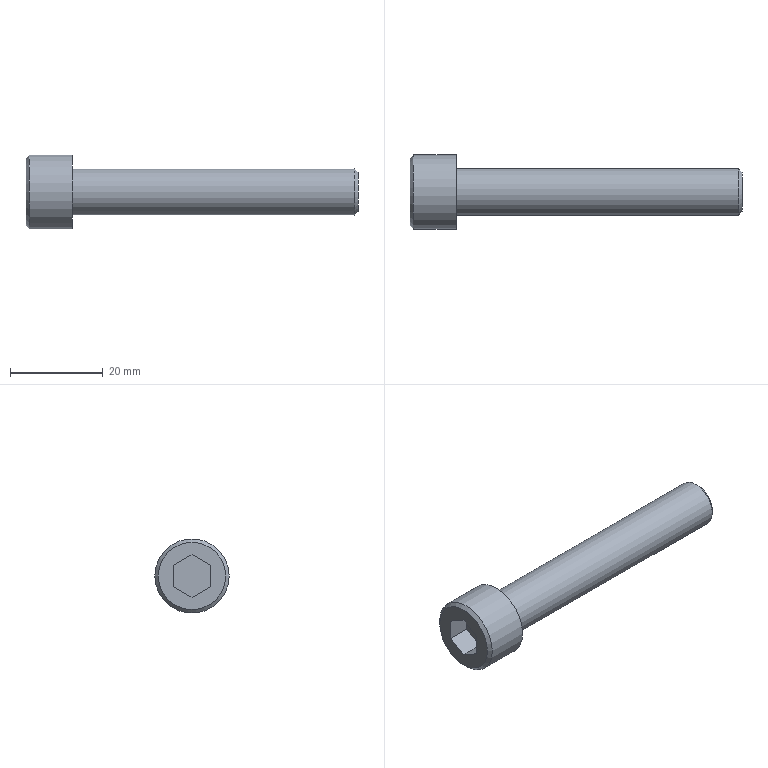Part | STEP file | solid 66 | 1 solid | 14 faces | box 71.5 x 16 x 16 mm | volume 6542 mm3 | plane 10 | cone 2 | cylinder 2 | commonest cylinder face diameters 10 x1 16 x1